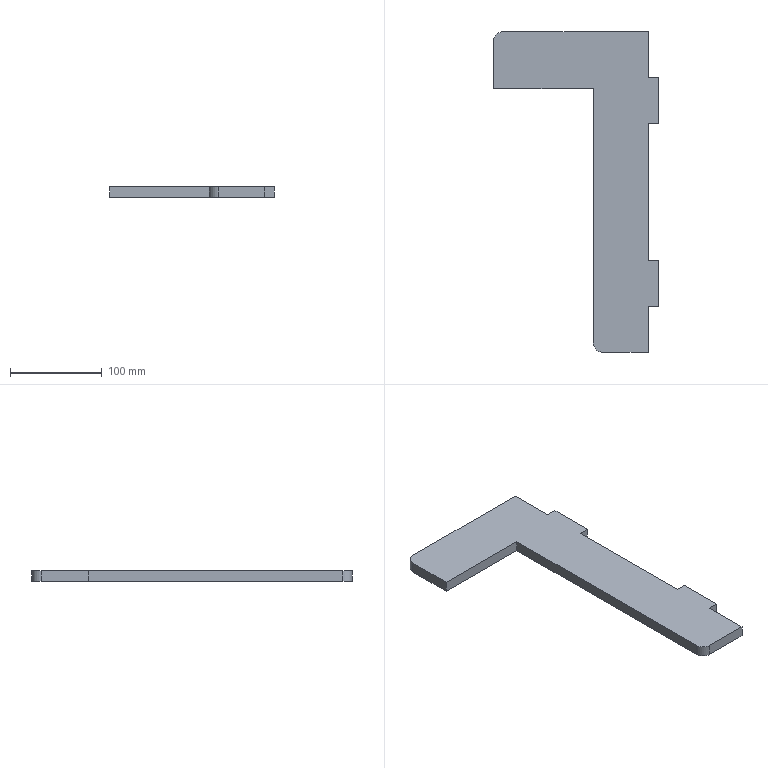Part | SolidWorks | features Fillet 1, FlatPattern 1, SMBaseFlange 1, SheetMetal 1 | 1 solid | 18 faces | box 180 x 350 x 12 mm | volume 345781 mm3 | plane 16 | cylinder 2 | commonest cylinder face diameters 20 x2
STEP:
#1=CARTESIAN_POINT('',(-1266.431,49.312,0.));
#2=VERTEX_POINT('',#1);
#3=CARTESIAN_POINT('',(-1157.431,49.312,0.));
#4=VERTEX_POINT('',#3);
#5=CARTESIAN_POINT('',(-1157.431,49.312,0.));
#6=DIRECTION('',(1.,0.,0.));
#7=VECTOR('',#6,1000.);
#8=LINE('',#5,#7);
#9=EDGE_CURVE('',#2,#4,#8,.T.);
#10=ORIENTED_EDGE('',*,*,#9,.F.);
#11=CARTESIAN_POINT('',(-1266.431,49.312,-12.));
#12=VERTEX_POINT('',#11);
#13=CARTESIAN_POINT('',(-1266.431,49.312,-12.));
#14=DIRECTION('',(0.,0.,1.));
#15=VECTOR('',#14,1000.);
#16=LINE('',#13,#15);
#17=EDGE_CURVE('',#12,#2,#16,.T.);
#18=ORIENTED_EDGE('',*,*,#17,.F.);
#19=CARTESIAN_POINT('',(-1157.431,49.312,-12.));
#20=VERTEX_POINT('',#19);
#21=CARTESIAN_POINT('',(-1157.431,49.312,-12.));
#22=DIRECTION('',(1.,0.,0.));
#23=VECTOR('',#22,1000.);
#24=LINE('',#21,#23);
#25=EDGE_CURVE('',#12,#20,#24,.T.);
#26=ORIENTED_EDGE('',*,*,#25,.T.);
#27=CARTESIAN_POINT('',(-1157.431,49.312,-12.));
#28=DIRECTION('',(0.,0.,1.));
#29=VECTOR('',#28,1000.);
#30=LINE('',#27,#29);
#31=EDGE_CURVE('',#20,#4,#30,.T.);
#32=ORIENTED_EDGE('',*,*,#31,.T.);
#33=EDGE_LOOP('',(#10,#18,#26,#32));
#34=FACE_OUTER_BOUND('',#33,.T.);
#35=CARTESIAN_POINT('',(-1157.431,49.312,-12.));
#36=DIRECTION('',(0.,-1.,0.));
#37=DIRECTION('',(1.,0.,0.));
#38=AXIS2_PLACEMENT_3D('',#35,#36,#37);
#39=PLANE('',#38);
#40=ADVANCED_FACE('',(#34),#39,.T.);
#41=CARTESIAN_POINT('',(-1266.431,101.312,0.));
#42=VERTEX_POINT('',#41);
#43=CARTESIAN_POINT('',(-1266.431,49.312,0.));
#44=DIRECTION('',(0.,-1.,0.));
#45=VECTOR('',#44,1000.);
#46=LINE('',#43,#45);
#47=EDGE_CURVE('',#42,#2,#46,.T.);
#48=ORIENTED_EDGE('',*,*,#47,.F.);
#49=CARTESIAN_POINT('',(-1266.431,101.312,-12.));
#50=VERTEX_POINT('',#49);
#51=CARTESIAN_POINT('',(-1266.431,101.312,-12.));
#52=DIRECTION('',(0.,0.,-1.));
#53=VECTOR('',#52,1000.);
#54=LINE('',#51,#53);
#55=EDGE_CURVE('',#42,#50,#54,.T.);
#56=ORIENTED_EDGE('',*,*,#55,.T.);
#57=CARTESIAN_POINT('',(-1266.431,49.312,-12.));
#58=DIRECTION('',(0.,-1.,0.));
#59=VECTOR('',#58,1000.);
#60=LINE('',#57,#59);
#61=EDGE_CURVE('',#50,#12,#60,.T.);
#62=ORIENTED_EDGE('',*,*,#61,.T.);
#63=ORIENTED_EDGE('',*,*,#17,.T.);
#64=EDGE_LOOP('',(#48,#56,#62,#63));
#65=FACE_OUTER_BOUND('',#64,.T.);
#66=CARTESIAN_POINT('',(-1266.431,49.312,-12.));
#67=DIRECTION('',(-1.,0.,0.));
#68=DIRECTION('',(0.,0.,1.));
#69=AXIS2_PLACEMENT_3D('',#66,#67,#68);
#70=PLANE('',#69);
#71=ADVANCED_FACE('',(#65),#70,.T.);
#72=CARTESIAN_POINT('',(-1097.431,111.312,-12.));
#73=VERTEX_POINT('',#72);
#74=CARTESIAN_POINT('',(-1256.431,111.312,-12.));
#75=VERTEX_POINT('',#74);
#76=CARTESIAN_POINT('',(-1266.431,111.312,-12.));
#77=DIRECTION('',(-1.,0.,0.));
#78=VECTOR('',#77,1000.);
#79=LINE('',#76,#78);
#80=EDGE_CURVE('',#73,#75,#79,.T.);
#81=ORIENTED_EDGE('',*,*,#80,.T.);
#82=CARTESIAN_POINT('',(-1256.431,111.312,0.));
#83=VERTEX_POINT('',#82);
#84=CARTESIAN_POINT('',(-1256.431,111.312,-12.));
#85=DIRECTION('',(0.,0.,1.));
#86=VECTOR('',#85,1000.);
#87=LINE('',#84,#86);
#88=EDGE_CURVE('',#75,#83,#87,.T.);
#89=ORIENTED_EDGE('',*,*,#88,.T.);
#90=CARTESIAN_POINT('',(-1097.431,111.312,0.));
#91=VERTEX_POINT('',#90);
#92=CARTESIAN_POINT('',(-1266.431,111.312,0.));
#93=DIRECTION('',(-1.,0.,0.));
#94=VECTOR('',#93,1000.);
#95=LINE('',#92,#94);
#96=EDGE_CURVE('',#91,#83,#95,.T.);
#97=ORIENTED_EDGE('',*,*,#96,.F.);
#98=CARTESIAN_POINT('',(-1097.431,111.312,-12.));
#99=DIRECTION('',(0.,0.,1.));
#100=VECTOR('',#99,1000.);
#101=LINE('',#98,#100);
#102=EDGE_CURVE('',#73,#91,#101,.T.);
#103=ORIENTED_EDGE('',*,*,#102,.F.);
#104=EDGE_LOOP('',(#81,#89,#97,#103));
#105=FACE_OUTER_BOUND('',#104,.T.);
#106=CARTESIAN_POINT('',(-1266.431,111.312,-12.));
#107=DIRECTION('',(0.,1.,0.));
#108=DIRECTION('',(0.,0.,1.));
#109=AXIS2_PLACEMENT_3D('',#106,#107,#108);
#110=PLANE('',#109);
#111=ADVANCED_FACE('',(#105),#110,.T.);
#112=CARTESIAN_POINT('',(-1097.431,61.312,0.));
#113=VERTEX_POINT('',#112);
#114=CARTESIAN_POINT('',(-1097.431,111.312,0.));
#115=DIRECTION('',(0.,1.,0.));
#116=VECTOR('',#115,1000.);
#117=LINE('',#114,#116);
#118=EDGE_CURVE('',#113,#91,#117,.T.);
#119=ORIENTED_EDGE('',*,*,#118,.F.);
#120=CARTESIAN_POINT('',(-1097.431,61.312,-12.));
#121=VERTEX_POINT('',#120);
#122=CARTESIAN_POINT('',(-1097.431,61.312,-12.));
#123=DIRECTION('',(0.,0.,1.));
#124=VECTOR('',#123,1000.);
#125=LINE('',#122,#124);
#126=EDGE_CURVE('',#121,#113,#125,.T.);
#127=ORIENTED_EDGE('',*,*,#126,.F.);
#128=CARTESIAN_POINT('',(-1097.431,111.312,-12.));
#129=DIRECTION('',(0.,1.,0.));
#130=VECTOR('',#129,1000.);
#131=LINE('',#128,#130);
#132=EDGE_CURVE('',#121,#73,#131,.T.);
#133=ORIENTED_EDGE('',*,*,#132,.T.);
#134=ORIENTED_EDGE('',*,*,#102,.T.);
#135=EDGE_LOOP('',(#119,#127,#133,#134));
#136=FACE_OUTER_BOUND('',#135,.T.);
#137=CARTESIAN_POINT('',(-1097.431,111.312,-12.));
#138=DIRECTION('',(1.,0.,0.));
#139=DIRECTION('',(0.,0.,-1.));
#140=AXIS2_PLACEMENT_3D('',#137,#138,#139);
#141=PLANE('',#140);
#142=ADVANCED_FACE('',(#136),#141,.T.);
#143=CARTESIAN_POINT('',(-1086.431,61.312,0.));
#144=VERTEX_POINT('',#143);
#145=CARTESIAN_POINT('',(-1097.431,61.312,0.));
#146=DIRECTION('',(-1.,0.,0.));
#147=VECTOR('',#146,1000.);
#148=LINE('',#145,#147);
#149=EDGE_CURVE('',#144,#113,#148,.T.);
#150=ORIENTED_EDGE('',*,*,#149,.F.);
#151=CARTESIAN_POINT('',(-1086.431,61.312,-12.));
#152=VERTEX_POINT('',#151);
#153=CARTESIAN_POINT('',(-1086.431,61.312,-12.));
#154=DIRECTION('',(0.,0.,1.));
#155=VECTOR('',#154,1000.);
#156=LINE('',#153,#155);
#157=EDGE_CURVE('',#152,#144,#156,.T.);
#158=ORIENTED_EDGE('',*,*,#157,.F.);
#159=CARTESIAN_POINT('',(-1097.431,61.312,-12.));
#160=DIRECTION('',(-1.,0.,0.));
#161=VECTOR('',#160,1000.);
#162=LINE('',#159,#161);
#163=EDGE_CURVE('',#152,#121,#162,.T.);
#164=ORIENTED_EDGE('',*,*,#163,.T.);
#165=ORIENTED_EDGE('',*,*,#126,.T.);
#166=EDGE_LOOP('',(#150,#158,#164,#165));
#167=FACE_OUTER_BOUND('',#166,.T.);
#168=CARTESIAN_POINT('',(-1097.431,61.312,-12.));
#169=DIRECTION('',(0.,1.,0.));
#170=DIRECTION('',(0.,0.,1.));
#171=AXIS2_PLACEMENT_3D('',#168,#169,#170);
#172=PLANE('',#171);
#173=ADVANCED_FACE('',(#167),#172,.T.);
#174=CARTESIAN_POINT('',(-1086.431,11.312,0.));
#175=VERTEX_POINT('',#174);
#176=CARTESIAN_POINT('',(-1086.431,61.312,0.));
#177=DIRECTION('',(0.,1.,0.));
#178=VECTOR('',#177,1000.);
#179=LINE('',#176,#178);
#180=EDGE_CURVE('',#175,#144,#179,.T.);
#181=ORIENTED_EDGE('',*,*,#180,.F.);
#182=CARTESIAN_POINT('',(-1086.431,11.312,-12.));
#183=VERTEX_POINT('',#182);
#184=CARTESIAN_POINT('',(-1086.431,11.312,-12.));
#185=DIRECTION('',(0.,0.,1.));
#186=VECTOR('',#185,1000.);
#187=LINE('',#184,#186);
#188=EDGE_CURVE('',#183,#175,#187,.T.);
#189=ORIENTED_EDGE('',*,*,#188,.F.);
#190=CARTESIAN_POINT('',(-1086.431,61.312,-12.));
#191=DIRECTION('',(0.,1.,0.));
#192=VECTOR('',#191,1000.);
#193=LINE('',#190,#192);
#194=EDGE_CURVE('',#183,#152,#193,.T.);
#195=ORIENTED_EDGE('',*,*,#194,.T.);
#196=ORIENTED_EDGE('',*,*,#157,.T.);
#197=EDGE_LOOP('',(#181,#189,#195,#196));
#198=FACE_OUTER_BOUND('',#197,.T.);
#199=CARTESIAN_POINT('',(-1086.431,61.312,-12.));
#200=DIRECTION('',(1.,0.,0.));
#201=DIRECTION('',(0.,0.,-1.));
#202=AXIS2_PLACEMENT_3D('',#199,#200,#201);
#203=PLANE('',#202);
#204=ADVANCED_FACE('',(#198),#203,.T.);
#205=CARTESIAN_POINT('',(-1097.431,11.312,0.));
#206=VERTEX_POINT('',#205);
#207=CARTESIAN_POINT('',(-1086.431,11.312,0.));
#208=DIRECTION('',(1.,0.,0.));
#209=VECTOR('',#208,1000.);
#210=LINE('',#207,#209);
#211=EDGE_CURVE('',#206,#175,#210,.T.);
#212=ORIENTED_EDGE('',*,*,#211,.F.);
#213=CARTESIAN_POINT('',(-1097.431,11.312,-12.));
#214=VERTEX_POINT('',#213);
#215=CARTESIAN_POINT('',(-1097.431,11.312,-12.));
#216=DIRECTION('',(0.,0.,1.));
#217=VECTOR('',#216,1000.);
#218=LINE('',#215,#217);
#219=EDGE_CURVE('',#214,#206,#218,.T.);
#220=ORIENTED_EDGE('',*,*,#219,.F.);
#221=CARTESIAN_POINT('',(-1086.431,11.312,-12.));
#222=DIRECTION('',(1.,0.,0.));
#223=VECTOR('',#222,1000.);
#224=LINE('',#221,#223);
#225=EDGE_CURVE('',#214,#183,#224,.T.);
#226=ORIENTED_EDGE('',*,*,#225,.T.);
#227=ORIENTED_EDGE('',*,*,#188,.T.);
#228=EDGE_LOOP('',(#212,#220,#226,#227));
#229=FACE_OUTER_BOUND('',#228,.T.);
#230=CARTESIAN_POINT('',(-1086.431,11.312,-12.));
#231=DIRECTION('',(0.,-1.,0.));
#232=DIRECTION('',(1.,0.,0.));
#233=AXIS2_PLACEMENT_3D('',#230,#231,#232);
#234=PLANE('',#233);
#235=ADVANCED_FACE('',(#229),#234,.T.);
#236=CARTESIAN_POINT('',(-1097.431,-138.688,0.));
#237=VERTEX_POINT('',#236);
#238=CARTESIAN_POINT('',(-1097.431,11.312,0.));
#239=DIRECTION('',(0.,1.,0.));
#240=VECTOR('',#239,1000.);
#241=LINE('',#238,#240);
#242=EDGE_CURVE('',#237,#206,#241,.T.);
#243=ORIENTED_EDGE('',*,*,#242,.F.);
#244=CARTESIAN_POINT('',(-1097.431,-138.688,-12.));
#245=VERTEX_POINT('',#244);
#246=CARTESIAN_POINT('',(-1097.431,-138.688,-12.));
#247=DIRECTION('',(0.,0.,1.));
#248=VECTOR('',#247,1000.);
#249=LINE('',#246,#248);
#250=EDGE_CURVE('',#245,#237,#249,.T.);
#251=ORIENTED_EDGE('',*,*,#250,.F.);
#252=CARTESIAN_POINT('',(-1097.431,11.312,-12.));
#253=DIRECTION('',(0.,1.,0.));
#254=VECTOR('',#253,1000.);
#255=LINE('',#252,#254);
#256=EDGE_CURVE('',#245,#214,#255,.T.);
#257=ORIENTED_EDGE('',*,*,#256,.T.);
#258=ORIENTED_EDGE('',*,*,#219,.T.);
#259=EDGE_LOOP('',(#243,#251,#257,#258));
#260=FACE_OUTER_BOUND('',#259,.T.);
#261=CARTESIAN_POINT('',(-1097.431,11.312,-12.));
#262=DIRECTION('',(1.,0.,0.));
#263=DIRECTION('',(0.,0.,-1.));
#264=AXIS2_PLACEMENT_3D('',#261,#262,#263);
#265=PLANE('',#264);
#266=ADVANCED_FACE('',(#260),#265,.T.);
#267=CARTESIAN_POINT('',(-1086.431,-138.688,0.));
#268=VERTEX_POINT('',#267);
#269=CARTESIAN_POINT('',(-1086.431,-138.688,0.));
#270=DIRECTION('',(-1.,0.,0.));
#271=VECTOR('',#270,1000.);
#272=LINE('',#269,#271);
#273=EDGE_CURVE('',#268,#237,#272,.T.);
#274=ORIENTED_EDGE('',*,*,#273,.F.);
#275=CARTESIAN_POINT('',(-1086.431,-138.688,-12.));
#276=VERTEX_POINT('',#275);
#277=CARTESIAN_POINT('',(-1086.431,-138.688,-12.));
#278=DIRECTION('',(0.,0.,1.));
#279=VECTOR('',#278,1000.);
#280=LINE('',#277,#279);
#281=EDGE_CURVE('',#276,#268,#280,.T.);
#282=ORIENTED_EDGE('',*,*,#281,.F.);
#283=CARTESIAN_POINT('',(-1086.431,-138.688,-12.));
#284=DIRECTION('',(-1.,0.,0.));
#285=VECTOR('',#284,1000.);
#286=LINE('',#283,#285);
#287=EDGE_CURVE('',#276,#245,#286,.T.);
#288=ORIENTED_EDGE('',*,*,#287,.T.);
#289=ORIENTED_EDGE('',*,*,#250,.T.);
#290=EDGE_LOOP('',(#274,#282,#288,#289));
#291=FACE_OUTER_BOUND('',#290,.T.);
#292=CARTESIAN_POINT('',(-1086.431,-138.688,-12.));
#293=DIRECTION('',(0.,1.,0.));
#294=DIRECTION('',(0.,0.,1.));
#295=AXIS2_PLACEMENT_3D('',#292,#293,#294);
#296=PLANE('',#295);
#297=ADVANCED_FACE('',(#291),#296,.T.);
#298=CARTESIAN_POINT('',(-1086.431,-188.688,0.));
#299=VERTEX_POINT('',#298);
#300=CARTESIAN_POINT('',(-1086.431,-188.688,0.));
#301=DIRECTION('',(0.,1.,0.));
#302=VECTOR('',#301,1000.);
#303=LINE('',#300,#302);
#304=EDGE_CURVE('',#299,#268,#303,.T.);
#305=ORIENTED_EDGE('',*,*,#304,.F.);
#306=CARTESIAN_POINT('',(-1086.431,-188.688,-12.));
#307=VERTEX_POINT('',#306);
#308=CARTESIAN_POINT('',(-1086.431,-188.688,-12.));
#309=DIRECTION('',(0.,0.,1.));
#310=VECTOR('',#309,1000.);
#311=LINE('',#308,#310);
#312=EDGE_CURVE('',#307,#299,#311,.T.);
#313=ORIENTED_EDGE('',*,*,#312,.F.);
#314=CARTESIAN_POINT('',(-1086.431,-188.688,-12.));
#315=DIRECTION('',(0.,1.,0.));
#316=VECTOR('',#315,1000.);
#317=LINE('',#314,#316);
#318=EDGE_CURVE('',#307,#276,#317,.T.);
#319=ORIENTED_EDGE('',*,*,#318,.T.);
#320=ORIENTED_EDGE('',*,*,#281,.T.);
#321=EDGE_LOOP('',(#305,#313,#319,#320));
#322=FACE_OUTER_BOUND('',#321,.T.);
#323=CARTESIAN_POINT('',(-1086.431,-188.688,-12.));
#324=DIRECTION('',(1.,0.,0.));
#325=DIRECTION('',(0.,0.,-1.));
#326=AXIS2_PLACEMENT_3D('',#323,#324,#325);
#327=PLANE('',#326);
#328=ADVANCED_FACE('',(#322),#327,.T.);
#329=CARTESIAN_POINT('',(-1097.431,-188.688,0.));
#330=VERTEX_POINT('',#329);
#331=CARTESIAN_POINT('',(-1097.431,-188.688,0.));
#332=DIRECTION('',(1.,0.,0.));
#333=VECTOR('',#332,1000.);
#334=LINE('',#331,#333);
#335=EDGE_CURVE('',#330,#299,#334,.T.);
#336=ORIENTED_EDGE('',*,*,#335,.F.);
#337=CARTESIAN_POINT('',(-1097.431,-188.688,-12.));
#338=VERTEX_POINT('',#337);
#339=CARTESIAN_POINT('',(-1097.431,-188.688,-12.));
#340=DIRECTION('',(0.,0.,1.));
#341=VECTOR('',#340,1000.);
#342=LINE('',#339,#341);
#343=EDGE_CURVE('',#338,#330,#342,.T.);
#344=ORIENTED_EDGE('',*,*,#343,.F.);
#345=CARTESIAN_POINT('',(-1097.431,-188.688,-12.));
#346=DIRECTION('',(1.,0.,0.));
#347=VECTOR('',#346,1000.);
#348=LINE('',#345,#347);
#349=EDGE_CURVE('',#338,#307,#348,.T.);
#350=ORIENTED_EDGE('',*,*,#349,.T.);
#351=ORIENTED_EDGE('',*,*,#312,.T.);
#352=EDGE_LOOP('',(#336,#344,#350,#351));
#353=FACE_OUTER_BOUND('',#352,.T.);
#354=CARTESIAN_POINT('',(-1097.431,-188.688,-12.));
#355=DIRECTION('',(0.,-1.,0.));
#356=DIRECTION('',(0.,0.,-1.));
#357=AXIS2_PLACEMENT_3D('',#354,#355,#356);
#358=PLANE('',#357);
#359=ADVANCED_FACE('',(#353),#358,.T.);
#360=CARTESIAN_POINT('',(-1097.431,-238.688,0.));
#361=VERTEX_POINT('',#360);
#362=CARTESIAN_POINT('',(-1097.431,-188.688,0.));
#363=DIRECTION('',(0.,1.,0.));
#364=VECTOR('',#363,1000.);
#365=LINE('',#362,#364);
#366=EDGE_CURVE('',#361,#330,#365,.T.);
#367=ORIENTED_EDGE('',*,*,#366,.F.);
#368=CARTESIAN_POINT('',(-1097.431,-238.688,-12.));
#369=VERTEX_POINT('',#368);
#370=CARTESIAN_POINT('',(-1097.431,-238.688,-12.));
#371=DIRECTION('',(0.,0.,1.));
#372=VECTOR('',#371,1000.);
#373=LINE('',#370,#372);
#374=EDGE_CURVE('',#369,#361,#373,.T.);
#375=ORIENTED_EDGE('',*,*,#374,.F.);
#376=CARTESIAN_POINT('',(-1097.431,-188.688,-12.));
#377=DIRECTION('',(0.,1.,0.));
#378=VECTOR('',#377,1000.);
#379=LINE('',#376,#378);
#380=EDGE_CURVE('',#369,#338,#379,.T.);
#381=ORIENTED_EDGE('',*,*,#380,.T.);
#382=ORIENTED_EDGE('',*,*,#343,.T.);
#383=EDGE_LOOP('',(#367,#375,#381,#382));
#384=FACE_OUTER_BOUND('',#383,.T.);
#385=CARTESIAN_POINT('',(-1097.431,-188.688,-12.));
#386=DIRECTION('',(1.,0.,0.));
#387=DIRECTION('',(0.,0.,-1.));
#388=AXIS2_PLACEMENT_3D('',#385,#386,#387);
#389=PLANE('',#388);
#390=ADVANCED_FACE('',(#384),#389,.T.);
#391=CARTESIAN_POINT('',(-1147.431,-238.688,0.));
#392=VERTEX_POINT('',#391);
#393=CARTESIAN_POINT('',(-1097.431,-238.688,0.));
#394=DIRECTION('',(1.,0.,0.));
#395=VECTOR('',#394,1000.);
#396=LINE('',#393,#395);
#397=EDGE_CURVE('',#392,#361,#396,.T.);
#398=ORIENTED_EDGE('',*,*,#397,.F.);
#399=CARTESIAN_POINT('',(-1147.431,-238.688,-12.));
#400=VERTEX_POINT('',#399);
#401=CARTESIAN_POINT('',(-1147.431,-238.688,-12.));
#402=DIRECTION('',(0.,0.,-1.));
#403=VECTOR('',#402,1000.);
#404=LINE('',#401,#403);
#405=EDGE_CURVE('',#392,#400,#404,.T.);
#406=ORIENTED_EDGE('',*,*,#405,.T.);
#407=CARTESIAN_POINT('',(-1097.431,-238.688,-12.));
#408=DIRECTION('',(1.,0.,0.));
#409=VECTOR('',#408,1000.);
#410=LINE('',#407,#409);
#411=EDGE_CURVE('',#400,#369,#410,.T.);
#412=ORIENTED_EDGE('',*,*,#411,.T.);
#413=ORIENTED_EDGE('',*,*,#374,.T.);
#414=EDGE_LOOP('',(#398,#406,#412,#413));
#415=FACE_OUTER_BOUND('',#414,.T.);
#416=CARTESIAN_POINT('',(-1097.431,-238.688,-12.));
#417=DIRECTION('',(0.,-1.,0.));
#418=DIRECTION('',(0.,0.,-1.));
#419=AXIS2_PLACEMENT_3D('',#416,#417,#418);
#420=PLANE('',#419);
#421=ADVANCED_FACE('',(#415),#420,.T.);
#422=CARTESIAN_POINT('',(-1157.431,-228.688,-12.));
#423=VERTEX_POINT('',#422);
#424=CARTESIAN_POINT('',(-1157.431,49.312,-12.));
#425=DIRECTION('',(0.,-1.,0.));
#426=VECTOR('',#425,1000.);
#427=LINE('',#424,#426);
#428=EDGE_CURVE('',#20,#423,#427,.T.);
#429=ORIENTED_EDGE('',*,*,#428,.T.);
#430=CARTESIAN_POINT('',(-1157.431,-228.688,0.));
#431=VERTEX_POINT('',#430);
#432=CARTESIAN_POINT('',(-1157.431,-228.688,-12.));
#433=DIRECTION('',(0.,0.,1.));
#434=VECTOR('',#433,1000.);
#435=LINE('',#432,#434);
#436=EDGE_CURVE('',#423,#431,#435,.T.);
#437=ORIENTED_EDGE('',*,*,#436,.T.);
#438=CARTESIAN_POINT('',(-1157.431,49.312,0.));
#439=DIRECTION('',(0.,-1.,0.));
#440=VECTOR('',#439,1000.);
#441=LINE('',#438,#440);
#442=EDGE_CURVE('',#4,#431,#441,.T.);
#443=ORIENTED_EDGE('',*,*,#442,.F.);
#444=ORIENTED_EDGE('',*,*,#31,.F.);
#445=EDGE_LOOP('',(#429,#437,#443,#444));
#446=FACE_OUTER_BOUND('',#445,.T.);
#447=CARTESIAN_POINT('',(-1157.431,49.312,-12.));
#448=DIRECTION('',(-1.,0.,0.));
#449=DIRECTION('',(0.,0.,1.));
#450=AXIS2_PLACEMENT_3D('',#447,#448,#449);
#451=PLANE('',#450);
#452=ADVANCED_FACE('',(#446),#451,.T.);
#453=ORIENTED_EDGE('',*,*,#61,.F.);
#454=CARTESIAN_POINT('',(-1256.431,101.312,-12.));
#455=DIRECTION('',(0.,0.,-1.));
#456=DIRECTION('',(-1.,0.,0.));
#457=AXIS2_PLACEMENT_3D('',#454,#455,#456);
#458=CIRCLE('',#457,10.);
#459=EDGE_CURVE('',#50,#75,#458,.T.);
#460=ORIENTED_EDGE('',*,*,#459,.T.);
#461=ORIENTED_EDGE('',*,*,#80,.F.);
#462=ORIENTED_EDGE('',*,*,#132,.F.);
#463=ORIENTED_EDGE('',*,*,#163,.F.);
#464=ORIENTED_EDGE('',*,*,#194,.F.);
#465=ORIENTED_EDGE('',*,*,#225,.F.);
#466=ORIENTED_EDGE('',*,*,#256,.F.);
#467=ORIENTED_EDGE('',*,*,#287,.F.);
#468=ORIENTED_EDGE('',*,*,#318,.F.);
#469=ORIENTED_EDGE('',*,*,#349,.F.);
#470=ORIENTED_EDGE('',*,*,#380,.F.);
#471=ORIENTED_EDGE('',*,*,#411,.F.);
#472=CARTESIAN_POINT('',(-1147.431,-228.688,-12.));
#473=DIRECTION('',(0.,0.,-1.));
#474=DIRECTION('',(-1.,0.,0.));
#475=AXIS2_PLACEMENT_3D('',#472,#473,#474);
#476=CIRCLE('',#475,10.);
#477=EDGE_CURVE('',#400,#423,#476,.T.);
#478=ORIENTED_EDGE('',*,*,#477,.T.);
#479=ORIENTED_EDGE('',*,*,#428,.F.);
#480=ORIENTED_EDGE('',*,*,#25,.F.);
#481=EDGE_LOOP('',(#453,#460,#461,#462,#463,#464,#465,#466,#467,#468,#469,#470,#471,#478,#479,#480));
#482=FACE_OUTER_BOUND('',#481,.T.);
#483=CARTESIAN_POINT('',(0.,0.,-12.));
#484=DIRECTION('',(0.,0.,-1.));
#485=DIRECTION('',(-1.,0.,0.));
#486=AXIS2_PLACEMENT_3D('',#483,#484,#485);
#487=PLANE('',#486);
#488=ADVANCED_FACE('',(#482),#487,.T.);
#489=ORIENTED_EDGE('',*,*,#96,.T.);
#490=CARTESIAN_POINT('',(-1256.431,101.312,0.));
#491=DIRECTION('',(0.,0.,1.));
#492=DIRECTION('',(-1.,0.,0.));
#493=AXIS2_PLACEMENT_3D('',#490,#491,#492);
#494=CIRCLE('',#493,10.);
#495=EDGE_CURVE('',#83,#42,#494,.T.);
#496=ORIENTED_EDGE('',*,*,#495,.T.);
#497=ORIENTED_EDGE('',*,*,#47,.T.);
#498=ORIENTED_EDGE('',*,*,#9,.T.);
#499=ORIENTED_EDGE('',*,*,#442,.T.);
#500=CARTESIAN_POINT('',(-1147.431,-228.688,0.));
#501=DIRECTION('',(0.,0.,1.));
#502=DIRECTION('',(-1.,0.,0.));
#503=AXIS2_PLACEMENT_3D('',#500,#501,#502);
#504=CIRCLE('',#503,10.);
#505=EDGE_CURVE('',#431,#392,#504,.T.);
#506=ORIENTED_EDGE('',*,*,#505,.T.);
#507=ORIENTED_EDGE('',*,*,#397,.T.);
#508=ORIENTED_EDGE('',*,*,#366,.T.);
#509=ORIENTED_EDGE('',*,*,#335,.T.);
#510=ORIENTED_EDGE('',*,*,#304,.T.);
#511=ORIENTED_EDGE('',*,*,#273,.T.);
#512=ORIENTED_EDGE('',*,*,#242,.T.);
#513=ORIENTED_EDGE('',*,*,#211,.T.);
#514=ORIENTED_EDGE('',*,*,#180,.T.);
#515=ORIENTED_EDGE('',*,*,#149,.T.);
#516=ORIENTED_EDGE('',*,*,#118,.T.);
#517=EDGE_LOOP('',(#489,#496,#497,#498,#499,#506,#507,#508,#509,#510,#511,#512,#513,#514,#515,#516));
#518=FACE_OUTER_BOUND('',#517,.T.);
#519=CARTESIAN_POINT('',(0.,0.,0.));
#520=DIRECTION('',(0.,0.,-1.));
#521=DIRECTION('',(-1.,0.,0.));
#522=AXIS2_PLACEMENT_3D('',#519,#520,#521);
#523=PLANE('',#522);
#524=ADVANCED_FACE('',(#518),#523,.F.);
#525=ORIENTED_EDGE('',*,*,#459,.F.);
#526=ORIENTED_EDGE('',*,*,#55,.F.);
#527=ORIENTED_EDGE('',*,*,#495,.F.);
#528=ORIENTED_EDGE('',*,*,#88,.F.);
#529=EDGE_LOOP('',(#525,#526,#527,#528));
#530=FACE_OUTER_BOUND('',#529,.T.);
#531=CARTESIAN_POINT('',(-1256.431,101.312,-12.));
#532=DIRECTION('',(0.,0.,1.));
#533=DIRECTION('',(1.,0.,0.));
#534=AXIS2_PLACEMENT_3D('',#531,#532,#533);
#535=CYLINDRICAL_SURFACE('',#534,10.);
#536=ADVANCED_FACE('',(#530),#535,.T.);
#537=ORIENTED_EDGE('',*,*,#477,.F.);
#538=ORIENTED_EDGE('',*,*,#405,.F.);
#539=ORIENTED_EDGE('',*,*,#505,.F.);
#540=ORIENTED_EDGE('',*,*,#436,.F.);
#541=EDGE_LOOP('',(#537,#538,#539,#540));
#542=FACE_OUTER_BOUND('',#541,.T.);
#543=CARTESIAN_POINT('',(-1147.431,-228.688,-12.));
#544=DIRECTION('',(0.,0.,1.));
#545=DIRECTION('',(1.,0.,0.));
#546=AXIS2_PLACEMENT_3D('',#543,#544,#545);
#547=CYLINDRICAL_SURFACE('',#546,10.);
#548=ADVANCED_FACE('',(#542),#547,.T.);
#549=CLOSED_SHELL('',(#40,#71,#111,#142,#173,#204,#235,#266,#297,#328,#359,#390,#421,#452,#488,#524,#536,#548));
#550=MANIFOLD_SOLID_BREP('',#549);
#551=CARTESIAN_POINT('',(0.,0.,0.));
#552=DIRECTION('',(0.,0.,1.));
#553=DIRECTION('',(1.,0.,0.));
#554=AXIS2_PLACEMENT_3D('',#551,#552,#553);
#555=(LENGTH_UNIT()NAMED_UNIT(*)SI_UNIT(.MILLI.,.METRE.));
#556=UNCERTAINTY_MEASURE_WITH_UNIT(LENGTH_MEASURE(0.00001),#555,'','');
#557=(NAMED_UNIT(*)PLANE_ANGLE_UNIT()SI_UNIT($,.RADIAN.));
#558=(NAMED_UNIT(*)SI_UNIT($,.STERADIAN.)SOLID_ANGLE_UNIT());
#559=(GEOMETRIC_REPRESENTATION_CONTEXT(3)GLOBAL_UNCERTAINTY_ASSIGNED_CONTEXT((#556))GLOBAL_UNIT_ASSIGNED_CONTEXT((#555,#557,#558))REPRESENTATION_CONTEXT('',''));
#560=ADVANCED_BREP_SHAPE_REPRESENTATION('',(#550,#554),#559);